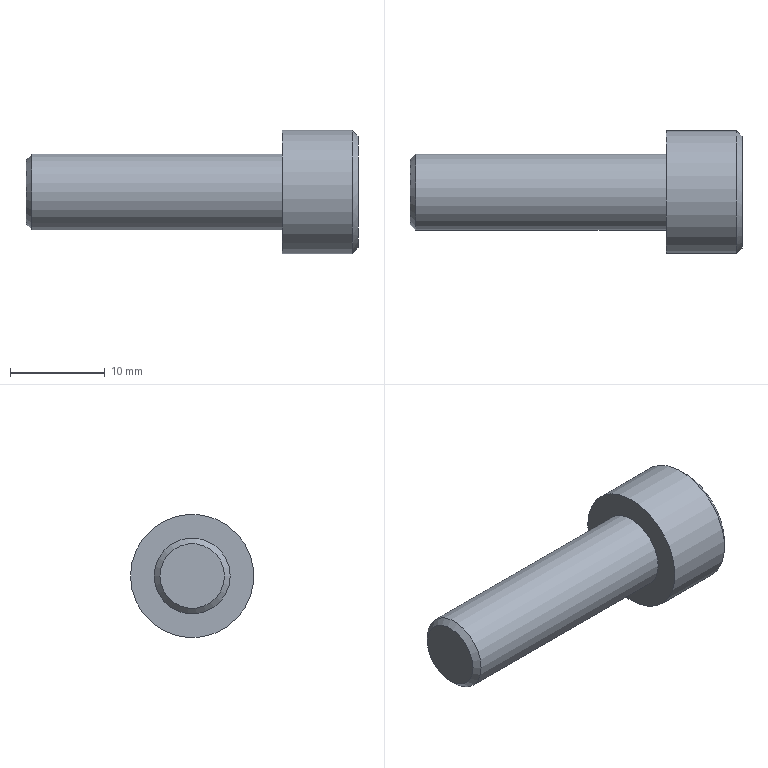Part | STEP file | solid 209 | 1 solid | 14 faces | box 35 x 13 x 13 mm | volume 2283 mm3 | plane 10 | cylinder 2 | cone 2 | commonest cylinder face diameters 8 x1 13 x1